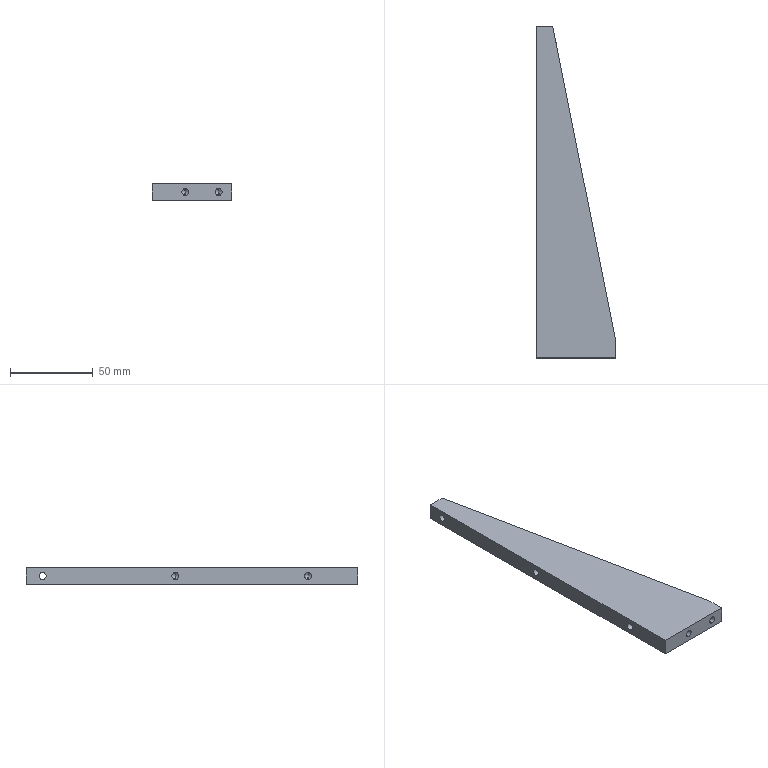Part | STEP file | 2070 Bag feed reinforcing rib 1 | 1 solid | 25 faces | box 48 x 200 x 10 mm | volume 58935 mm3 | cylinder 10 | cone 8 | plane 7 | commonest cylinder face diameters 4.2 x10